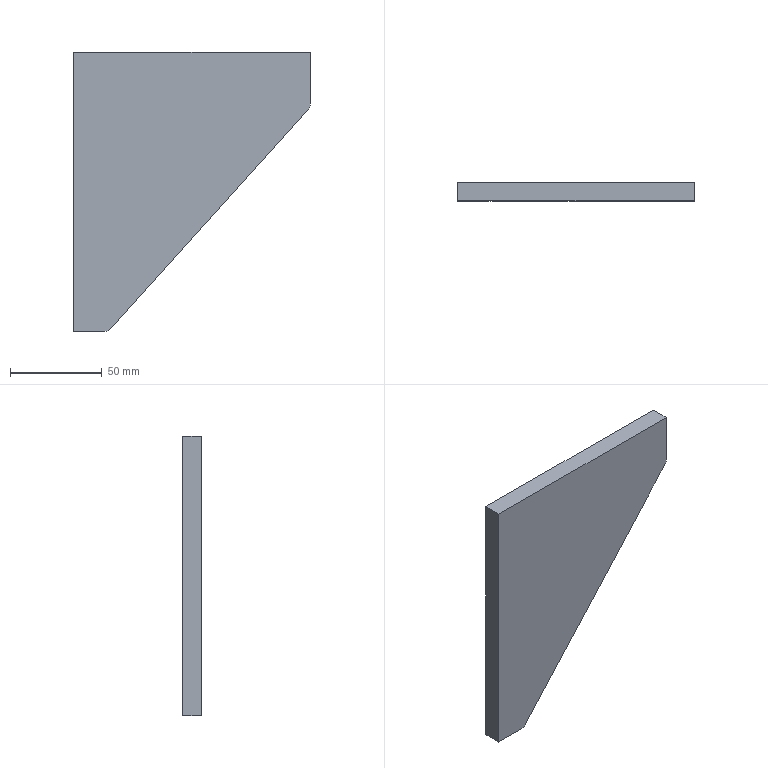Part | SolidWorks | features DeleteBody 1, MBimport 1 | 1 solid | 9 faces | box 129 x 10 x 152 mm | volume 128824 mm3 | plane 7 | cylinder 2 | commonest cylinder face diameters 8.922 x1 9 x1
STEP:
#1=CARTESIAN_POINT('',(501.,-304.5,-990.5));
#2=VERTEX_POINT('',#1);
#3=CARTESIAN_POINT('',(501.,-304.5,-1142.5));
#4=VERTEX_POINT('',#3);
#5=CARTESIAN_POINT('',(501.,-304.5,-1142.5));
#6=DIRECTION('',(0.,0.,-1.));
#7=VECTOR('',#6,1000.);
#8=LINE('',#5,#7);
#9=EDGE_CURVE('',#2,#4,#8,.T.);
#10=ORIENTED_EDGE('',*,*,#9,.T.);
#11=CARTESIAN_POINT('',(517.969,-304.5,-1142.5));
#12=VERTEX_POINT('',#11);
#13=CARTESIAN_POINT('',(517.969,-304.5,-1142.5));
#14=DIRECTION('',(1.,0.,0.));
#15=VECTOR('',#14,1000.);
#16=LINE('',#13,#15);
#17=EDGE_CURVE('',#4,#12,#16,.T.);
#18=ORIENTED_EDGE('',*,*,#17,.T.);
#19=CARTESIAN_POINT('',(521.284,-304.5,-1141.024));
#20=VERTEX_POINT('',#19);
#21=CARTESIAN_POINT('',(517.969,-304.5,-1138.039));
#22=DIRECTION('',(0.,-1.,0.));
#23=DIRECTION('',(-1.,0.,0.));
#24=AXIS2_PLACEMENT_3D('',#21,#22,#23);
#25=CIRCLE('',#24,4.461);
#26=EDGE_CURVE('',#12,#20,#25,.T.);
#27=ORIENTED_EDGE('',*,*,#26,.T.);
#28=CARTESIAN_POINT('',(628.844,-304.5,-1021.566));
#29=VERTEX_POINT('',#28);
#30=CARTESIAN_POINT('',(628.844,-304.5,-1021.566));
#31=DIRECTION('',(0.6691,0.,0.7431));
#32=VECTOR('',#31,1000.);
#33=LINE('',#30,#32);
#34=EDGE_CURVE('',#20,#29,#33,.T.);
#35=ORIENTED_EDGE('',*,*,#34,.T.);
#36=CARTESIAN_POINT('',(630.,-304.5,-1018.555));
#37=VERTEX_POINT('',#36);
#38=CARTESIAN_POINT('',(625.5,-304.5,-1018.555));
#39=DIRECTION('',(0.,-1.,0.));
#40=DIRECTION('',(-1.,0.,0.));
#41=AXIS2_PLACEMENT_3D('',#38,#39,#40);
#42=CIRCLE('',#41,4.5);
#43=EDGE_CURVE('',#29,#37,#42,.T.);
#44=ORIENTED_EDGE('',*,*,#43,.T.);
#45=CARTESIAN_POINT('',(630.,-304.5,-990.5));
#46=VERTEX_POINT('',#45);
#47=CARTESIAN_POINT('',(630.,-304.5,-990.5));
#48=DIRECTION('',(0.,0.,1.));
#49=VECTOR('',#48,1000.);
#50=LINE('',#47,#49);
#51=EDGE_CURVE('',#37,#46,#50,.T.);
#52=ORIENTED_EDGE('',*,*,#51,.T.);
#53=CARTESIAN_POINT('',(501.,-304.5,-990.5));
#54=DIRECTION('',(-1.,0.,0.));
#55=VECTOR('',#54,1000.);
#56=LINE('',#53,#55);
#57=EDGE_CURVE('',#46,#2,#56,.T.);
#58=ORIENTED_EDGE('',*,*,#57,.T.);
#59=EDGE_LOOP('',(#10,#18,#27,#35,#44,#52,#58));
#60=FACE_OUTER_BOUND('',#59,.T.);
#61=CARTESIAN_POINT('',(625.5,-304.5,-1018.555));
#62=DIRECTION('',(0.,-1.,0.));
#63=DIRECTION('',(0.,0.,-1.));
#64=AXIS2_PLACEMENT_3D('',#61,#62,#63);
#65=PLANE('',#64);
#66=ADVANCED_FACE('',(#60),#65,.T.);
#67=CARTESIAN_POINT('',(501.,-294.5,-990.5));
#68=VERTEX_POINT('',#67);
#69=CARTESIAN_POINT('',(501.,-294.5,-1142.5));
#70=VERTEX_POINT('',#69);
#71=CARTESIAN_POINT('',(501.,-294.5,-1142.5));
#72=DIRECTION('',(0.,0.,-1.));
#73=VECTOR('',#72,1000.);
#74=LINE('',#71,#73);
#75=EDGE_CURVE('',#68,#70,#74,.T.);
#76=ORIENTED_EDGE('',*,*,#75,.F.);
#77=CARTESIAN_POINT('',(630.,-294.5,-990.5));
#78=VERTEX_POINT('',#77);
#79=CARTESIAN_POINT('',(501.,-294.5,-990.5));
#80=DIRECTION('',(-1.,0.,0.));
#81=VECTOR('',#80,1000.);
#82=LINE('',#79,#81);
#83=EDGE_CURVE('',#78,#68,#82,.T.);
#84=ORIENTED_EDGE('',*,*,#83,.F.);
#85=CARTESIAN_POINT('',(630.,-294.5,-1018.555));
#86=VERTEX_POINT('',#85);
#87=CARTESIAN_POINT('',(630.,-294.5,-990.5));
#88=DIRECTION('',(0.,0.,1.));
#89=VECTOR('',#88,1000.);
#90=LINE('',#87,#89);
#91=EDGE_CURVE('',#86,#78,#90,.T.);
#92=ORIENTED_EDGE('',*,*,#91,.F.);
#93=CARTESIAN_POINT('',(628.844,-294.5,-1021.566));
#94=VERTEX_POINT('',#93);
#95=CARTESIAN_POINT('',(625.5,-294.5,-1018.555));
#96=DIRECTION('',(0.,-1.,0.));
#97=DIRECTION('',(-1.,0.,0.));
#98=AXIS2_PLACEMENT_3D('',#95,#96,#97);
#99=CIRCLE('',#98,4.5);
#100=EDGE_CURVE('',#94,#86,#99,.T.);
#101=ORIENTED_EDGE('',*,*,#100,.F.);
#102=CARTESIAN_POINT('',(521.284,-294.5,-1141.024));
#103=VERTEX_POINT('',#102);
#104=CARTESIAN_POINT('',(628.844,-294.5,-1021.566));
#105=DIRECTION('',(0.6691,0.,0.7431));
#106=VECTOR('',#105,1000.);
#107=LINE('',#104,#106);
#108=EDGE_CURVE('',#103,#94,#107,.T.);
#109=ORIENTED_EDGE('',*,*,#108,.F.);
#110=CARTESIAN_POINT('',(517.969,-294.5,-1142.5));
#111=VERTEX_POINT('',#110);
#112=CARTESIAN_POINT('',(517.969,-294.5,-1138.039));
#113=DIRECTION('',(0.,-1.,0.));
#114=DIRECTION('',(-1.,0.,0.));
#115=AXIS2_PLACEMENT_3D('',#112,#113,#114);
#116=CIRCLE('',#115,4.461);
#117=EDGE_CURVE('',#111,#103,#116,.T.);
#118=ORIENTED_EDGE('',*,*,#117,.F.);
#119=CARTESIAN_POINT('',(517.969,-294.5,-1142.5));
#120=DIRECTION('',(1.,0.,0.));
#121=VECTOR('',#120,1000.);
#122=LINE('',#119,#121);
#123=EDGE_CURVE('',#70,#111,#122,.T.);
#124=ORIENTED_EDGE('',*,*,#123,.F.);
#125=EDGE_LOOP('',(#76,#84,#92,#101,#109,#118,#124));
#126=FACE_OUTER_BOUND('',#125,.T.);
#127=CARTESIAN_POINT('',(625.5,-294.5,-1018.555));
#128=DIRECTION('',(0.,-1.,0.));
#129=DIRECTION('',(0.,0.,-1.));
#130=AXIS2_PLACEMENT_3D('',#127,#128,#129);
#131=PLANE('',#130);
#132=ADVANCED_FACE('',(#126),#131,.F.);
#133=ORIENTED_EDGE('',*,*,#17,.F.);
#134=CARTESIAN_POINT('',(501.,-294.5,-1142.5));
#135=DIRECTION('',(0.,1.,0.));
#136=VECTOR('',#135,1000.);
#137=LINE('',#134,#136);
#138=EDGE_CURVE('',#4,#70,#137,.T.);
#139=ORIENTED_EDGE('',*,*,#138,.T.);
#140=ORIENTED_EDGE('',*,*,#123,.T.);
#141=CARTESIAN_POINT('',(517.969,-294.5,-1142.5));
#142=DIRECTION('',(0.,1.,0.));
#143=VECTOR('',#142,1000.);
#144=LINE('',#141,#143);
#145=EDGE_CURVE('',#12,#111,#144,.T.);
#146=ORIENTED_EDGE('',*,*,#145,.F.);
#147=EDGE_LOOP('',(#133,#139,#140,#146));
#148=FACE_OUTER_BOUND('',#147,.T.);
#149=CARTESIAN_POINT('',(517.969,-294.5,-1142.5));
#150=DIRECTION('',(0.,0.,-1.));
#151=DIRECTION('',(0.,-1.,0.));
#152=AXIS2_PLACEMENT_3D('',#149,#150,#151);
#153=PLANE('',#152);
#154=ADVANCED_FACE('',(#148),#153,.T.);
#155=ORIENTED_EDGE('',*,*,#26,.F.);
#156=ORIENTED_EDGE('',*,*,#145,.T.);
#157=ORIENTED_EDGE('',*,*,#117,.T.);
#158=CARTESIAN_POINT('',(521.284,-294.5,-1141.024));
#159=DIRECTION('',(0.,1.,0.));
#160=VECTOR('',#159,1000.);
#161=LINE('',#158,#160);
#162=EDGE_CURVE('',#20,#103,#161,.T.);
#163=ORIENTED_EDGE('',*,*,#162,.F.);
#164=EDGE_LOOP('',(#155,#156,#157,#163));
#165=FACE_OUTER_BOUND('',#164,.T.);
#166=CARTESIAN_POINT('',(517.969,-294.5,-1138.039));
#167=DIRECTION('',(0.,-1.,0.));
#168=DIRECTION('',(0.,0.,1.));
#169=AXIS2_PLACEMENT_3D('',#166,#167,#168);
#170=CYLINDRICAL_SURFACE('',#169,4.461);
#171=ADVANCED_FACE('',(#165),#170,.T.);
#172=ORIENTED_EDGE('',*,*,#34,.F.);
#173=ORIENTED_EDGE('',*,*,#162,.T.);
#174=ORIENTED_EDGE('',*,*,#108,.T.);
#175=CARTESIAN_POINT('',(628.844,-294.5,-1021.566));
#176=DIRECTION('',(0.,1.,0.));
#177=VECTOR('',#176,1000.);
#178=LINE('',#175,#177);
#179=EDGE_CURVE('',#29,#94,#178,.T.);
#180=ORIENTED_EDGE('',*,*,#179,.F.);
#181=EDGE_LOOP('',(#172,#173,#174,#180));
#182=FACE_OUTER_BOUND('',#181,.T.);
#183=CARTESIAN_POINT('',(628.844,-294.5,-1021.566));
#184=DIRECTION('',(0.7431,0.,-0.6691));
#185=DIRECTION('',(0.,-1.,0.));
#186=AXIS2_PLACEMENT_3D('',#183,#184,#185);
#187=PLANE('',#186);
#188=ADVANCED_FACE('',(#182),#187,.T.);
#189=ORIENTED_EDGE('',*,*,#43,.F.);
#190=ORIENTED_EDGE('',*,*,#179,.T.);
#191=ORIENTED_EDGE('',*,*,#100,.T.);
#192=CARTESIAN_POINT('',(630.,-294.5,-1018.555));
#193=DIRECTION('',(0.,1.,0.));
#194=VECTOR('',#193,1000.);
#195=LINE('',#192,#194);
#196=EDGE_CURVE('',#37,#86,#195,.T.);
#197=ORIENTED_EDGE('',*,*,#196,.F.);
#198=EDGE_LOOP('',(#189,#190,#191,#197));
#199=FACE_OUTER_BOUND('',#198,.T.);
#200=CARTESIAN_POINT('',(625.5,-294.5,-1018.555));
#201=DIRECTION('',(0.,-1.,0.));
#202=DIRECTION('',(0.,0.,1.));
#203=AXIS2_PLACEMENT_3D('',#200,#201,#202);
#204=CYLINDRICAL_SURFACE('',#203,4.5);
#205=ADVANCED_FACE('',(#199),#204,.T.);
#206=ORIENTED_EDGE('',*,*,#51,.F.);
#207=ORIENTED_EDGE('',*,*,#196,.T.);
#208=ORIENTED_EDGE('',*,*,#91,.T.);
#209=CARTESIAN_POINT('',(630.,-294.5,-990.5));
#210=DIRECTION('',(0.,1.,0.));
#211=VECTOR('',#210,1000.);
#212=LINE('',#209,#211);
#213=EDGE_CURVE('',#46,#78,#212,.T.);
#214=ORIENTED_EDGE('',*,*,#213,.F.);
#215=EDGE_LOOP('',(#206,#207,#208,#214));
#216=FACE_OUTER_BOUND('',#215,.T.);
#217=CARTESIAN_POINT('',(630.,-294.5,-990.5));
#218=DIRECTION('',(1.,0.,0.));
#219=DIRECTION('',(0.,1.,0.));
#220=AXIS2_PLACEMENT_3D('',#217,#218,#219);
#221=PLANE('',#220);
#222=ADVANCED_FACE('',(#216),#221,.T.);
#223=ORIENTED_EDGE('',*,*,#57,.F.);
#224=ORIENTED_EDGE('',*,*,#213,.T.);
#225=ORIENTED_EDGE('',*,*,#83,.T.);
#226=CARTESIAN_POINT('',(501.,-294.5,-990.5));
#227=DIRECTION('',(0.,1.,0.));
#228=VECTOR('',#227,1000.);
#229=LINE('',#226,#228);
#230=EDGE_CURVE('',#2,#68,#229,.T.);
#231=ORIENTED_EDGE('',*,*,#230,.F.);
#232=EDGE_LOOP('',(#223,#224,#225,#231));
#233=FACE_OUTER_BOUND('',#232,.T.);
#234=CARTESIAN_POINT('',(501.,-294.5,-990.5));
#235=DIRECTION('',(0.,0.,1.));
#236=DIRECTION('',(1.,0.,0.));
#237=AXIS2_PLACEMENT_3D('',#234,#235,#236);
#238=PLANE('',#237);
#239=ADVANCED_FACE('',(#233),#238,.T.);
#240=ORIENTED_EDGE('',*,*,#9,.F.);
#241=ORIENTED_EDGE('',*,*,#230,.T.);
#242=ORIENTED_EDGE('',*,*,#75,.T.);
#243=ORIENTED_EDGE('',*,*,#138,.F.);
#244=EDGE_LOOP('',(#240,#241,#242,#243));
#245=FACE_OUTER_BOUND('',#244,.T.);
#246=CARTESIAN_POINT('',(501.,-294.5,-1142.5));
#247=DIRECTION('',(-1.,0.,0.));
#248=DIRECTION('',(0.,1.,0.));
#249=AXIS2_PLACEMENT_3D('',#246,#247,#248);
#250=PLANE('',#249);
#251=ADVANCED_FACE('',(#245),#250,.T.);
#252=CLOSED_SHELL('',(#66,#132,#154,#171,#188,#205,#222,#239,#251));
#253=MANIFOLD_SOLID_BREP('',#252);
#254=CARTESIAN_POINT('',(0.,0.,0.));
#255=DIRECTION('',(0.,0.,1.));
#256=DIRECTION('',(1.,0.,0.));
#257=AXIS2_PLACEMENT_3D('',#254,#255,#256);
#258=(LENGTH_UNIT()NAMED_UNIT(*)SI_UNIT(.MILLI.,.METRE.));
#259=UNCERTAINTY_MEASURE_WITH_UNIT(LENGTH_MEASURE(0.00001),#258,'','');
#260=(NAMED_UNIT(*)PLANE_ANGLE_UNIT()SI_UNIT($,.RADIAN.));
#261=(NAMED_UNIT(*)SI_UNIT($,.STERADIAN.)SOLID_ANGLE_UNIT());
#262=(GEOMETRIC_REPRESENTATION_CONTEXT(3)GLOBAL_UNCERTAINTY_ASSIGNED_CONTEXT((#259))GLOBAL_UNIT_ASSIGNED_CONTEXT((#258,#260,#261))REPRESENTATION_CONTEXT('',''));
#263=ADVANCED_BREP_SHAPE_REPRESENTATION('',(#253,#257),#262);